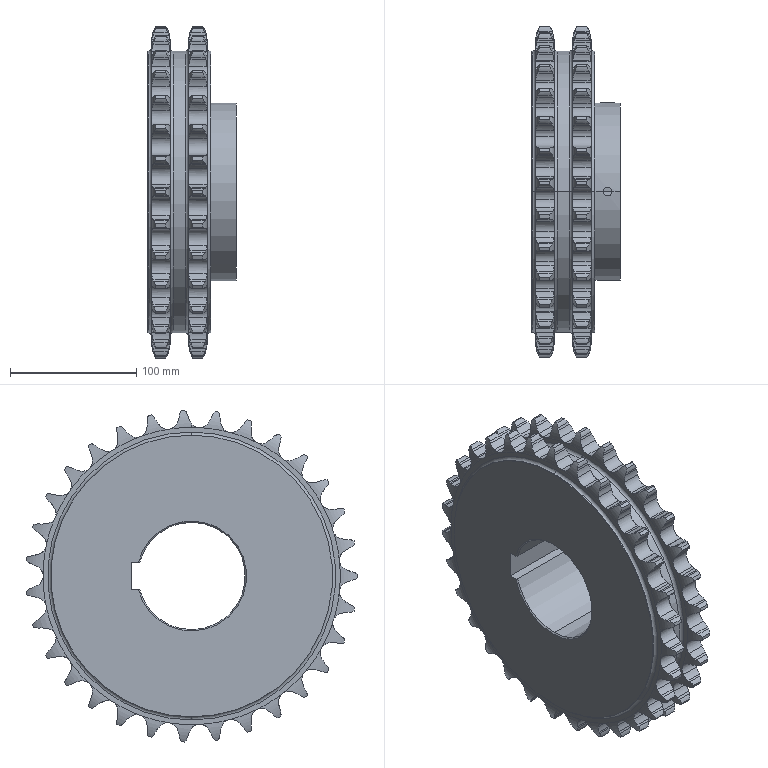Part | SolidWorks | features Revolution 3, Chamfer 2, Cut 2, ICE 2, CirPattern 1, LPattern 1 | 1 solid | 695 faces | box 70 x 262.456 x 262.787 mm | volume 2093366 mm3 | cylinder 419 | torus 136 | plane 134 | cone 6 | commonest cylinder face diameters 22.826 x132 41.467 x130 16.059 x80 263 x62 223 x6 6.8 x4